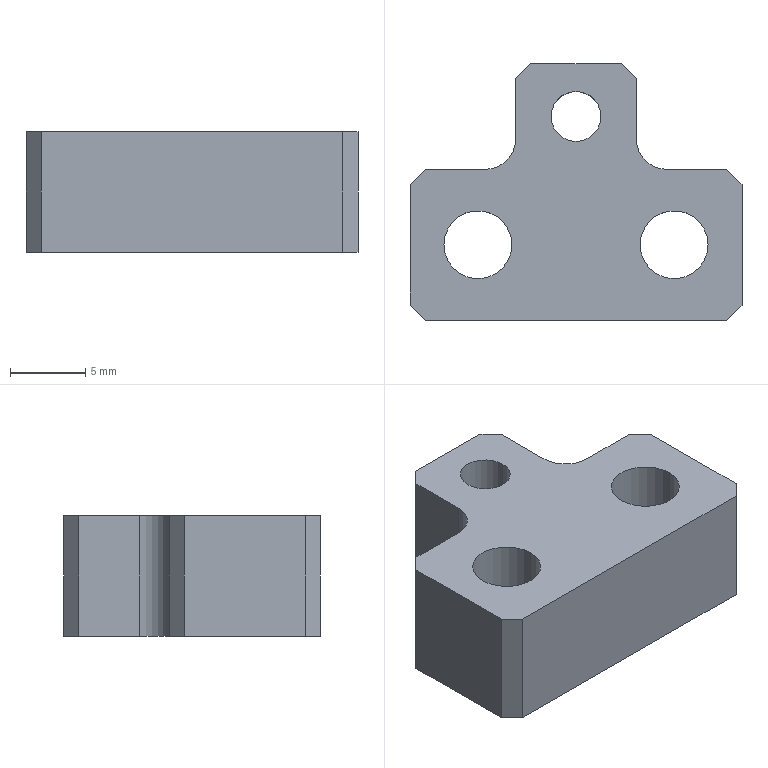Part | SolidWorks | features HoleWzd 2, Chamfer 1, Extrusion 1, Fillet 1, ICE 1 | 1 solid | 30 faces | box 22 x 17 x 8 mm | volume 1559 mm3 | plane 18 | cylinder 12 | commonest cylinder face diameters 4.5 x4 8 x4 3.3 x2 4 x2
STEP:
#1=CARTESIAN_POINT('',(1.65,8.5,8.));
#2=VERTEX_POINT('',#1);
#3=CARTESIAN_POINT('',(-1.65,8.5,8.));
#4=VERTEX_POINT('',#3);
#5=CARTESIAN_POINT('',(0.,8.5,8.));
#6=DIRECTION('',(0.,0.,-1.));
#7=DIRECTION('',(-1.,0.,0.));
#8=AXIS2_PLACEMENT_3D('',#5,#6,#7);
#9=CIRCLE('',#8,1.65);
#10=EDGE_CURVE('',#2,#4,#9,.T.);
#11=ORIENTED_EDGE('',*,*,#10,.F.);
#12=CARTESIAN_POINT('',(1.65,8.5,0.));
#13=VERTEX_POINT('',#12);
#14=CARTESIAN_POINT('',(1.65,8.5,0.));
#15=DIRECTION('',(0.,0.,-1.));
#16=VECTOR('',#15,1000.);
#17=LINE('',#14,#16);
#18=EDGE_CURVE('',#2,#13,#17,.T.);
#19=ORIENTED_EDGE('',*,*,#18,.T.);
#20=CARTESIAN_POINT('',(-1.65,8.5,0.));
#21=VERTEX_POINT('',#20);
#22=CARTESIAN_POINT('',(0.,8.5,0.));
#23=DIRECTION('',(0.,0.,-1.));
#24=DIRECTION('',(-1.,0.,0.));
#25=AXIS2_PLACEMENT_3D('',#22,#23,#24);
#26=CIRCLE('',#25,1.65);
#27=EDGE_CURVE('',#13,#21,#26,.T.);
#28=ORIENTED_EDGE('',*,*,#27,.T.);
#29=CARTESIAN_POINT('',(-1.65,8.5,0.));
#30=DIRECTION('',(0.,0.,-1.));
#31=VECTOR('',#30,1000.);
#32=LINE('',#29,#31);
#33=EDGE_CURVE('',#4,#21,#32,.T.);
#34=ORIENTED_EDGE('',*,*,#33,.F.);
#35=EDGE_LOOP('',(#11,#19,#28,#34));
#36=FACE_OUTER_BOUND('',#35,.T.);
#37=CARTESIAN_POINT('',(0.,8.5,0.));
#38=DIRECTION('',(0.,0.,-1.));
#39=DIRECTION('',(-1.,0.,0.));
#40=AXIS2_PLACEMENT_3D('',#37,#38,#39);
#41=CYLINDRICAL_SURFACE('',#40,1.65);
#42=ADVANCED_FACE('',(#36),#41,.F.);
#43=CARTESIAN_POINT('',(10.5,0.,4.6));
#44=VERTEX_POINT('',#43);
#45=CARTESIAN_POINT('',(2.5,0.,4.6));
#46=VERTEX_POINT('',#45);
#47=CARTESIAN_POINT('',(6.5,0.,4.6));
#48=DIRECTION('',(0.,0.,-1.));
#49=DIRECTION('',(-1.,0.,0.));
#50=AXIS2_PLACEMENT_3D('',#47,#48,#49);
#51=CIRCLE('',#50,4.);
#52=EDGE_CURVE('',#44,#46,#51,.T.);
#53=ORIENTED_EDGE('',*,*,#52,.F.);
#54=CARTESIAN_POINT('',(10.5,0.,0.));
#55=VERTEX_POINT('',#54);
#56=CARTESIAN_POINT('',(10.5,0.,0.));
#57=DIRECTION('',(0.,0.,-1.));
#58=VECTOR('',#57,1000.);
#59=LINE('',#56,#58);
#60=EDGE_CURVE('',#44,#55,#59,.T.);
#61=ORIENTED_EDGE('',*,*,#60,.T.);
#62=CARTESIAN_POINT('',(2.5,0.,0.));
#63=VERTEX_POINT('',#62);
#64=CARTESIAN_POINT('',(6.5,0.,0.));
#65=DIRECTION('',(0.,0.,-1.));
#66=DIRECTION('',(-1.,0.,0.));
#67=AXIS2_PLACEMENT_3D('',#64,#65,#66);
#68=CIRCLE('',#67,4.);
#69=EDGE_CURVE('',#55,#63,#68,.T.);
#70=ORIENTED_EDGE('',*,*,#69,.T.);
#71=CARTESIAN_POINT('',(2.5,0.,0.));
#72=DIRECTION('',(0.,0.,-1.));
#73=VECTOR('',#72,1000.);
#74=LINE('',#71,#73);
#75=EDGE_CURVE('',#46,#63,#74,.T.);
#76=ORIENTED_EDGE('',*,*,#75,.F.);
#77=EDGE_LOOP('',(#53,#61,#70,#76));
#78=FACE_OUTER_BOUND('',#77,.T.);
#79=CARTESIAN_POINT('',(6.5,0.,0.));
#80=DIRECTION('',(0.,0.,-1.));
#81=DIRECTION('',(-1.,0.,0.));
#82=AXIS2_PLACEMENT_3D('',#79,#80,#81);
#83=CYLINDRICAL_SURFACE('',#82,4.);
#84=ADVANCED_FACE('',(#78),#83,.F.);
#85=CARTESIAN_POINT('',(8.75,0.,8.));
#86=VERTEX_POINT('',#85);
#87=CARTESIAN_POINT('',(4.25,0.,8.));
#88=VERTEX_POINT('',#87);
#89=CARTESIAN_POINT('',(6.5,0.,8.));
#90=DIRECTION('',(0.,0.,-1.));
#91=DIRECTION('',(-1.,0.,0.));
#92=AXIS2_PLACEMENT_3D('',#89,#90,#91);
#93=CIRCLE('',#92,2.25);
#94=EDGE_CURVE('',#86,#88,#93,.T.);
#95=ORIENTED_EDGE('',*,*,#94,.F.);
#96=CARTESIAN_POINT('',(8.75,0.,4.6));
#97=VERTEX_POINT('',#96);
#98=CARTESIAN_POINT('',(8.75,0.,0.));
#99=DIRECTION('',(0.,0.,-1.));
#100=VECTOR('',#99,1000.);
#101=LINE('',#98,#100);
#102=EDGE_CURVE('',#86,#97,#101,.T.);
#103=ORIENTED_EDGE('',*,*,#102,.T.);
#104=CARTESIAN_POINT('',(4.25,0.,4.6));
#105=VERTEX_POINT('',#104);
#106=CARTESIAN_POINT('',(6.5,0.,4.6));
#107=DIRECTION('',(0.,0.,-1.));
#108=DIRECTION('',(-1.,0.,0.));
#109=AXIS2_PLACEMENT_3D('',#106,#107,#108);
#110=CIRCLE('',#109,2.25);
#111=EDGE_CURVE('',#97,#105,#110,.T.);
#112=ORIENTED_EDGE('',*,*,#111,.T.);
#113=CARTESIAN_POINT('',(4.25,0.,0.));
#114=DIRECTION('',(0.,0.,-1.));
#115=VECTOR('',#114,1000.);
#116=LINE('',#113,#115);
#117=EDGE_CURVE('',#88,#105,#116,.T.);
#118=ORIENTED_EDGE('',*,*,#117,.F.);
#119=EDGE_LOOP('',(#95,#103,#112,#118));
#120=FACE_OUTER_BOUND('',#119,.T.);
#121=CARTESIAN_POINT('',(6.5,0.,0.));
#122=DIRECTION('',(0.,0.,-1.));
#123=DIRECTION('',(-1.,0.,0.));
#124=AXIS2_PLACEMENT_3D('',#121,#122,#123);
#125=CYLINDRICAL_SURFACE('',#124,2.25);
#126=ADVANCED_FACE('',(#120),#125,.F.);
#127=CARTESIAN_POINT('',(-2.5,0.,4.6));
#128=VERTEX_POINT('',#127);
#129=CARTESIAN_POINT('',(-10.5,0.,4.6));
#130=VERTEX_POINT('',#129);
#131=CARTESIAN_POINT('',(-6.5,0.,4.6));
#132=DIRECTION('',(0.,0.,-1.));
#133=DIRECTION('',(-1.,0.,0.));
#134=AXIS2_PLACEMENT_3D('',#131,#132,#133);
#135=CIRCLE('',#134,4.);
#136=EDGE_CURVE('',#128,#130,#135,.T.);
#137=ORIENTED_EDGE('',*,*,#136,.F.);
#138=CARTESIAN_POINT('',(-2.5,0.,0.));
#139=VERTEX_POINT('',#138);
#140=CARTESIAN_POINT('',(-2.5,0.,0.));
#141=DIRECTION('',(0.,0.,-1.));
#142=VECTOR('',#141,1000.);
#143=LINE('',#140,#142);
#144=EDGE_CURVE('',#128,#139,#143,.T.);
#145=ORIENTED_EDGE('',*,*,#144,.T.);
#146=CARTESIAN_POINT('',(-10.5,0.,0.));
#147=VERTEX_POINT('',#146);
#148=CARTESIAN_POINT('',(-6.5,0.,0.));
#149=DIRECTION('',(0.,0.,-1.));
#150=DIRECTION('',(-1.,0.,0.));
#151=AXIS2_PLACEMENT_3D('',#148,#149,#150);
#152=CIRCLE('',#151,4.);
#153=EDGE_CURVE('',#139,#147,#152,.T.);
#154=ORIENTED_EDGE('',*,*,#153,.T.);
#155=CARTESIAN_POINT('',(-10.5,0.,0.));
#156=DIRECTION('',(0.,0.,-1.));
#157=VECTOR('',#156,1000.);
#158=LINE('',#155,#157);
#159=EDGE_CURVE('',#130,#147,#158,.T.);
#160=ORIENTED_EDGE('',*,*,#159,.F.);
#161=EDGE_LOOP('',(#137,#145,#154,#160));
#162=FACE_OUTER_BOUND('',#161,.T.);
#163=CARTESIAN_POINT('',(-6.5,0.,0.));
#164=DIRECTION('',(0.,0.,-1.));
#165=DIRECTION('',(-1.,0.,0.));
#166=AXIS2_PLACEMENT_3D('',#163,#164,#165);
#167=CYLINDRICAL_SURFACE('',#166,4.);
#168=ADVANCED_FACE('',(#162),#167,.F.);
#169=CARTESIAN_POINT('',(-4.25,0.,8.));
#170=VERTEX_POINT('',#169);
#171=CARTESIAN_POINT('',(-8.75,0.,8.));
#172=VERTEX_POINT('',#171);
#173=CARTESIAN_POINT('',(-6.5,0.,8.));
#174=DIRECTION('',(0.,0.,-1.));
#175=DIRECTION('',(-1.,0.,0.));
#176=AXIS2_PLACEMENT_3D('',#173,#174,#175);
#177=CIRCLE('',#176,2.25);
#178=EDGE_CURVE('',#170,#172,#177,.T.);
#179=ORIENTED_EDGE('',*,*,#178,.F.);
#180=CARTESIAN_POINT('',(-4.25,0.,4.6));
#181=VERTEX_POINT('',#180);
#182=CARTESIAN_POINT('',(-4.25,0.,0.));
#183=DIRECTION('',(0.,0.,-1.));
#184=VECTOR('',#183,1000.);
#185=LINE('',#182,#184);
#186=EDGE_CURVE('',#170,#181,#185,.T.);
#187=ORIENTED_EDGE('',*,*,#186,.T.);
#188=CARTESIAN_POINT('',(-8.75,0.,4.6));
#189=VERTEX_POINT('',#188);
#190=CARTESIAN_POINT('',(-6.5,0.,4.6));
#191=DIRECTION('',(0.,0.,-1.));
#192=DIRECTION('',(-1.,0.,0.));
#193=AXIS2_PLACEMENT_3D('',#190,#191,#192);
#194=CIRCLE('',#193,2.25);
#195=EDGE_CURVE('',#181,#189,#194,.T.);
#196=ORIENTED_EDGE('',*,*,#195,.T.);
#197=CARTESIAN_POINT('',(-8.75,0.,0.));
#198=DIRECTION('',(0.,0.,-1.));
#199=VECTOR('',#198,1000.);
#200=LINE('',#197,#199);
#201=EDGE_CURVE('',#172,#189,#200,.T.);
#202=ORIENTED_EDGE('',*,*,#201,.F.);
#203=EDGE_LOOP('',(#179,#187,#196,#202));
#204=FACE_OUTER_BOUND('',#203,.T.);
#205=CARTESIAN_POINT('',(-6.5,0.,0.));
#206=DIRECTION('',(0.,0.,-1.));
#207=DIRECTION('',(-1.,0.,0.));
#208=AXIS2_PLACEMENT_3D('',#205,#206,#207);
#209=CYLINDRICAL_SURFACE('',#208,2.25);
#210=ADVANCED_FACE('',(#204),#209,.F.);
#211=CARTESIAN_POINT('',(10.,5.,8.));
#212=VERTEX_POINT('',#211);
#213=CARTESIAN_POINT('',(6.,5.,8.));
#214=VERTEX_POINT('',#213);
#215=CARTESIAN_POINT('',(-11.,5.,8.));
#216=DIRECTION('',(-1.,0.,0.));
#217=VECTOR('',#216,1000.);
#218=LINE('',#215,#217);
#219=EDGE_CURVE('',#212,#214,#218,.T.);
#220=ORIENTED_EDGE('',*,*,#219,.F.);
#221=CARTESIAN_POINT('',(10.,5.,0.));
#222=VERTEX_POINT('',#221);
#223=CARTESIAN_POINT('',(10.,5.,8.));
#224=DIRECTION('',(0.,0.,-1.));
#225=VECTOR('',#224,1000.);
#226=LINE('',#223,#225);
#227=EDGE_CURVE('',#212,#222,#226,.T.);
#228=ORIENTED_EDGE('',*,*,#227,.T.);
#229=CARTESIAN_POINT('',(6.,5.,0.));
#230=VERTEX_POINT('',#229);
#231=CARTESIAN_POINT('',(-11.,5.,0.));
#232=DIRECTION('',(-1.,0.,0.));
#233=VECTOR('',#232,1000.);
#234=LINE('',#231,#233);
#235=EDGE_CURVE('',#222,#230,#234,.T.);
#236=ORIENTED_EDGE('',*,*,#235,.T.);
#237=CARTESIAN_POINT('',(6.,5.,8.));
#238=DIRECTION('',(0.,0.,1.));
#239=VECTOR('',#238,1000.);
#240=LINE('',#237,#239);
#241=EDGE_CURVE('',#230,#214,#240,.T.);
#242=ORIENTED_EDGE('',*,*,#241,.T.);
#243=EDGE_LOOP('',(#220,#228,#236,#242));
#244=FACE_OUTER_BOUND('',#243,.T.);
#245=CARTESIAN_POINT('',(-11.,5.,8.));
#246=DIRECTION('',(0.,-1.,0.));
#247=DIRECTION('',(0.,0.,-1.));
#248=AXIS2_PLACEMENT_3D('',#245,#246,#247);
#249=PLANE('',#248);
#250=ADVANCED_FACE('',(#244),#249,.F.);
#251=CARTESIAN_POINT('',(11.,-4.,8.));
#252=VERTEX_POINT('',#251);
#253=CARTESIAN_POINT('',(11.,4.,8.));
#254=VERTEX_POINT('',#253);
#255=CARTESIAN_POINT('',(11.,5.,8.));
#256=DIRECTION('',(0.,1.,0.));
#257=VECTOR('',#256,1000.);
#258=LINE('',#255,#257);
#259=EDGE_CURVE('',#252,#254,#258,.T.);
#260=ORIENTED_EDGE('',*,*,#259,.F.);
#261=CARTESIAN_POINT('',(11.,-4.,0.));
#262=VERTEX_POINT('',#261);
#263=CARTESIAN_POINT('',(11.,-4.,8.));
#264=DIRECTION('',(0.,0.,-1.));
#265=VECTOR('',#264,1000.);
#266=LINE('',#263,#265);
#267=EDGE_CURVE('',#252,#262,#266,.T.);
#268=ORIENTED_EDGE('',*,*,#267,.T.);
#269=CARTESIAN_POINT('',(11.,4.,0.));
#270=VERTEX_POINT('',#269);
#271=CARTESIAN_POINT('',(11.,5.,0.));
#272=DIRECTION('',(0.,1.,0.));
#273=VECTOR('',#272,1000.);
#274=LINE('',#271,#273);
#275=EDGE_CURVE('',#262,#270,#274,.T.);
#276=ORIENTED_EDGE('',*,*,#275,.T.);
#277=CARTESIAN_POINT('',(11.,4.,8.));
#278=DIRECTION('',(0.,0.,1.));
#279=VECTOR('',#278,1000.);
#280=LINE('',#277,#279);
#281=EDGE_CURVE('',#270,#254,#280,.T.);
#282=ORIENTED_EDGE('',*,*,#281,.T.);
#283=EDGE_LOOP('',(#260,#268,#276,#282));
#284=FACE_OUTER_BOUND('',#283,.T.);
#285=CARTESIAN_POINT('',(11.,5.,8.));
#286=DIRECTION('',(-1.,0.,0.));
#287=DIRECTION('',(0.,0.,1.));
#288=AXIS2_PLACEMENT_3D('',#285,#286,#287);
#289=PLANE('',#288);
#290=ADVANCED_FACE('',(#284),#289,.F.);
#291=CARTESIAN_POINT('',(-6.,5.,0.));
#292=VERTEX_POINT('',#291);
#293=CARTESIAN_POINT('',(-10.,5.,0.));
#294=VERTEX_POINT('',#293);
#295=CARTESIAN_POINT('',(-11.,5.,0.));
#296=DIRECTION('',(-1.,0.,0.));
#297=VECTOR('',#296,1000.);
#298=LINE('',#295,#297);
#299=EDGE_CURVE('',#292,#294,#298,.T.);
#300=ORIENTED_EDGE('',*,*,#299,.T.);
#301=CARTESIAN_POINT('',(-10.,5.,8.));
#302=VERTEX_POINT('',#301);
#303=CARTESIAN_POINT('',(-10.,5.,8.));
#304=DIRECTION('',(0.,0.,1.));
#305=VECTOR('',#304,1000.);
#306=LINE('',#303,#305);
#307=EDGE_CURVE('',#294,#302,#306,.T.);
#308=ORIENTED_EDGE('',*,*,#307,.T.);
#309=CARTESIAN_POINT('',(-6.,5.,8.));
#310=VERTEX_POINT('',#309);
#311=CARTESIAN_POINT('',(-11.,5.,8.));
#312=DIRECTION('',(-1.,0.,0.));
#313=VECTOR('',#312,1000.);
#314=LINE('',#311,#313);
#315=EDGE_CURVE('',#310,#302,#314,.T.);
#316=ORIENTED_EDGE('',*,*,#315,.F.);
#317=CARTESIAN_POINT('',(-6.,5.,8.));
#318=DIRECTION('',(0.,0.,-1.));
#319=VECTOR('',#318,1000.);
#320=LINE('',#317,#319);
#321=EDGE_CURVE('',#310,#292,#320,.T.);
#322=ORIENTED_EDGE('',*,*,#321,.T.);
#323=EDGE_LOOP('',(#300,#308,#316,#322));
#324=FACE_OUTER_BOUND('',#323,.T.);
#325=CARTESIAN_POINT('',(-11.,5.,8.));
#326=DIRECTION('',(0.,-1.,0.));
#327=DIRECTION('',(0.,0.,-1.));
#328=AXIS2_PLACEMENT_3D('',#325,#326,#327);
#329=PLANE('',#328);
#330=ADVANCED_FACE('',(#324),#329,.F.);
#331=CARTESIAN_POINT('',(-11.,4.,8.));
#332=VERTEX_POINT('',#331);
#333=CARTESIAN_POINT('',(-11.,-4.,8.));
#334=VERTEX_POINT('',#333);
#335=CARTESIAN_POINT('',(-11.,5.,8.));
#336=DIRECTION('',(0.,-1.,0.));
#337=VECTOR('',#336,1000.);
#338=LINE('',#335,#337);
#339=EDGE_CURVE('',#332,#334,#338,.T.);
#340=ORIENTED_EDGE('',*,*,#339,.F.);
#341=CARTESIAN_POINT('',(-11.,4.,0.));
#342=VERTEX_POINT('',#341);
#343=CARTESIAN_POINT('',(-11.,4.,8.));
#344=DIRECTION('',(0.,0.,-1.));
#345=VECTOR('',#344,1000.);
#346=LINE('',#343,#345);
#347=EDGE_CURVE('',#332,#342,#346,.T.);
#348=ORIENTED_EDGE('',*,*,#347,.T.);
#349=CARTESIAN_POINT('',(-11.,-4.,0.));
#350=VERTEX_POINT('',#349);
#351=CARTESIAN_POINT('',(-11.,5.,0.));
#352=DIRECTION('',(0.,-1.,0.));
#353=VECTOR('',#352,1000.);
#354=LINE('',#351,#353);
#355=EDGE_CURVE('',#342,#350,#354,.T.);
#356=ORIENTED_EDGE('',*,*,#355,.T.);
#357=CARTESIAN_POINT('',(-11.,-4.,8.));
#358=DIRECTION('',(0.,0.,1.));
#359=VECTOR('',#358,1000.);
#360=LINE('',#357,#359);
#361=EDGE_CURVE('',#350,#334,#360,.T.);
#362=ORIENTED_EDGE('',*,*,#361,.T.);
#363=EDGE_LOOP('',(#340,#348,#356,#362));
#364=FACE_OUTER_BOUND('',#363,.T.);
#365=CARTESIAN_POINT('',(-11.,5.,8.));
#366=DIRECTION('',(1.,0.,0.));
#367=DIRECTION('',(0.,1.,0.));
#368=AXIS2_PLACEMENT_3D('',#365,#366,#367);
#369=PLANE('',#368);
#370=ADVANCED_FACE('',(#364),#369,.F.);
#371=CARTESIAN_POINT('',(-10.,-5.,0.));
#372=VERTEX_POINT('',#371);
#373=CARTESIAN_POINT('',(10.,-5.,0.));
#374=VERTEX_POINT('',#373);
#375=CARTESIAN_POINT('',(-11.,-5.,0.));
#376=DIRECTION('',(1.,0.,0.));
#377=VECTOR('',#376,1000.);
#378=LINE('',#375,#377);
#379=EDGE_CURVE('',#372,#374,#378,.T.);
#380=ORIENTED_EDGE('',*,*,#379,.T.);
#381=CARTESIAN_POINT('',(10.,-5.,8.));
#382=VERTEX_POINT('',#381);
#383=CARTESIAN_POINT('',(10.,-5.,8.));
#384=DIRECTION('',(0.,0.,1.));
#385=VECTOR('',#384,1000.);
#386=LINE('',#383,#385);
#387=EDGE_CURVE('',#374,#382,#386,.T.);
#388=ORIENTED_EDGE('',*,*,#387,.T.);
#389=CARTESIAN_POINT('',(-10.,-5.,8.));
#390=VERTEX_POINT('',#389);
#391=CARTESIAN_POINT('',(-11.,-5.,8.));
#392=DIRECTION('',(1.,0.,0.));
#393=VECTOR('',#392,1000.);
#394=LINE('',#391,#393);
#395=EDGE_CURVE('',#390,#382,#394,.T.);
#396=ORIENTED_EDGE('',*,*,#395,.F.);
#397=CARTESIAN_POINT('',(-10.,-5.,8.));
#398=DIRECTION('',(0.,0.,-1.));
#399=VECTOR('',#398,1000.);
#400=LINE('',#397,#399);
#401=EDGE_CURVE('',#390,#372,#400,.T.);
#402=ORIENTED_EDGE('',*,*,#401,.T.);
#403=EDGE_LOOP('',(#380,#388,#396,#402));
#404=FACE_OUTER_BOUND('',#403,.T.);
#405=CARTESIAN_POINT('',(-11.,-5.,8.));
#406=DIRECTION('',(0.,1.,0.));
#407=DIRECTION('',(0.,0.,1.));
#408=AXIS2_PLACEMENT_3D('',#405,#406,#407);
#409=PLANE('',#408);
#410=ADVANCED_FACE('',(#404),#409,.F.);
#411=CARTESIAN_POINT('',(0.,8.5,8.));
#412=DIRECTION('',(0.,0.,-1.));
#413=DIRECTION('',(-1.,0.,0.));
#414=AXIS2_PLACEMENT_3D('',#411,#412,#413);
#415=CIRCLE('',#414,1.65);
#416=EDGE_CURVE('',#4,#2,#415,.T.);
#417=ORIENTED_EDGE('',*,*,#416,.T.);
#418=ORIENTED_EDGE('',*,*,#10,.T.);
#419=EDGE_LOOP('',(#417,#418));
#420=FACE_BOUND('',#419,.T.);
#421=CARTESIAN_POINT('',(6.5,0.,8.));
#422=DIRECTION('',(0.,0.,-1.));
#423=DIRECTION('',(-1.,0.,0.));
#424=AXIS2_PLACEMENT_3D('',#421,#422,#423);
#425=CIRCLE('',#424,2.25);
#426=EDGE_CURVE('',#88,#86,#425,.T.);
#427=ORIENTED_EDGE('',*,*,#426,.T.);
#428=ORIENTED_EDGE('',*,*,#94,.T.);
#429=EDGE_LOOP('',(#427,#428));
#430=FACE_BOUND('',#429,.T.);
#431=CARTESIAN_POINT('',(-6.5,0.,8.));
#432=DIRECTION('',(0.,0.,-1.));
#433=DIRECTION('',(-1.,0.,0.));
#434=AXIS2_PLACEMENT_3D('',#431,#432,#433);
#435=CIRCLE('',#434,2.25);
#436=EDGE_CURVE('',#172,#170,#435,.T.);
#437=ORIENTED_EDGE('',*,*,#436,.T.);
#438=ORIENTED_EDGE('',*,*,#178,.T.);
#439=EDGE_LOOP('',(#437,#438));
#440=FACE_BOUND('',#439,.T.);
#441=ORIENTED_EDGE('',*,*,#395,.T.);
#442=CARTESIAN_POINT('',(7.5,-7.5,8.));
#443=DIRECTION('',(0.7071,0.7071,0.));
#444=VECTOR('',#443,1000.);
#445=LINE('',#442,#444);
#446=EDGE_CURVE('',#382,#252,#445,.T.);
#447=ORIENTED_EDGE('',*,*,#446,.T.);
#448=ORIENTED_EDGE('',*,*,#259,.T.);
#449=CARTESIAN_POINT('',(7.5,7.5,8.));
#450=DIRECTION('',(-0.7071,0.7071,0.));
#451=VECTOR('',#450,1000.);
#452=LINE('',#449,#451);
#453=EDGE_CURVE('',#254,#212,#452,.T.);
#454=ORIENTED_EDGE('',*,*,#453,.T.);
#455=ORIENTED_EDGE('',*,*,#219,.T.);
#456=CARTESIAN_POINT('',(4.,7.,8.));
#457=VERTEX_POINT('',#456);
#458=CARTESIAN_POINT('',(6.,7.,8.));
#459=DIRECTION('',(0.,0.,-1.));
#460=DIRECTION('',(1.,0.,0.));
#461=AXIS2_PLACEMENT_3D('',#458,#459,#460);
#462=CIRCLE('',#461,2.);
#463=EDGE_CURVE('',#214,#457,#462,.T.);
#464=ORIENTED_EDGE('',*,*,#463,.T.);
#465=CARTESIAN_POINT('',(4.,11.,8.));
#466=VERTEX_POINT('',#465);
#467=CARTESIAN_POINT('',(4.,5.,8.));
#468=DIRECTION('',(0.,-1.,0.));
#469=VECTOR('',#468,1000.);
#470=LINE('',#467,#469);
#471=EDGE_CURVE('',#466,#457,#470,.T.);
#472=ORIENTED_EDGE('',*,*,#471,.F.);
#473=CARTESIAN_POINT('',(3.,12.,8.));
#474=VERTEX_POINT('',#473);
#475=CARTESIAN_POINT('',(7.5,7.5,8.));
#476=DIRECTION('',(-0.7071,0.7071,0.));
#477=VECTOR('',#476,1000.);
#478=LINE('',#475,#477);
#479=EDGE_CURVE('',#466,#474,#478,.T.);
#480=ORIENTED_EDGE('',*,*,#479,.T.);
#481=CARTESIAN_POINT('',(-3.,12.,8.));
#482=VERTEX_POINT('',#481);
#483=CARTESIAN_POINT('',(4.,12.,8.));
#484=DIRECTION('',(1.,0.,0.));
#485=VECTOR('',#484,1000.);
#486=LINE('',#483,#485);
#487=EDGE_CURVE('',#482,#474,#486,.T.);
#488=ORIENTED_EDGE('',*,*,#487,.F.);
#489=CARTESIAN_POINT('',(-4.,11.,8.));
#490=VERTEX_POINT('',#489);
#491=CARTESIAN_POINT('',(-7.5,7.5,8.));
#492=DIRECTION('',(-0.7071,-0.7071,0.));
#493=VECTOR('',#492,1000.);
#494=LINE('',#491,#493);
#495=EDGE_CURVE('',#482,#490,#494,.T.);
#496=ORIENTED_EDGE('',*,*,#495,.T.);
#497=CARTESIAN_POINT('',(-4.,7.,8.));
#498=VERTEX_POINT('',#497);
#499=CARTESIAN_POINT('',(-4.,5.,8.));
#500=DIRECTION('',(0.,1.,0.));
#501=VECTOR('',#500,1000.);
#502=LINE('',#499,#501);
#503=EDGE_CURVE('',#498,#490,#502,.T.);
#504=ORIENTED_EDGE('',*,*,#503,.F.);
#505=CARTESIAN_POINT('',(-6.,7.,8.));
#506=DIRECTION('',(0.,0.,-1.));
#507=DIRECTION('',(1.,0.,0.));
#508=AXIS2_PLACEMENT_3D('',#505,#506,#507);
#509=CIRCLE('',#508,2.);
#510=EDGE_CURVE('',#498,#310,#509,.T.);
#511=ORIENTED_EDGE('',*,*,#510,.T.);
#512=ORIENTED_EDGE('',*,*,#315,.T.);
#513=CARTESIAN_POINT('',(-7.5,7.5,8.));
#514=DIRECTION('',(-0.7071,-0.7071,0.));
#515=VECTOR('',#514,1000.);
#516=LINE('',#513,#515);
#517=EDGE_CURVE('',#302,#332,#516,.T.);
#518=ORIENTED_EDGE('',*,*,#517,.T.);
#519=ORIENTED_EDGE('',*,*,#339,.T.);
#520=CARTESIAN_POINT('',(-7.5,-7.5,8.));
#521=DIRECTION('',(0.7071,-0.7071,0.));
#522=VECTOR('',#521,1000.);
#523=LINE('',#520,#522);
#524=EDGE_CURVE('',#334,#390,#523,.T.);
#525=ORIENTED_EDGE('',*,*,#524,.T.);
#526=EDGE_LOOP('',(#441,#447,#448,#454,#455,#464,#472,#480,#488,#496,#504,#511,#512,#518,#519,#525));
#527=FACE_OUTER_BOUND('',#526,.T.);
#528=CARTESIAN_POINT('',(0.,0.,8.));
#529=DIRECTION('',(0.,0.,1.));
#530=DIRECTION('',(1.,0.,0.));
#531=AXIS2_PLACEMENT_3D('',#528,#529,#530);
#532=PLANE('',#531);
#533=ADVANCED_FACE('',(#420,#430,#440,#527),#532,.T.);
#534=CARTESIAN_POINT('',(0.,8.5,0.));
#535=DIRECTION('',(0.,0.,-1.));
#536=DIRECTION('',(-1.,0.,0.));
#537=AXIS2_PLACEMENT_3D('',#534,#535,#536);
#538=CIRCLE('',#537,1.65);
#539=EDGE_CURVE('',#21,#13,#538,.T.);
#540=ORIENTED_EDGE('',*,*,#539,.F.);
#541=ORIENTED_EDGE('',*,*,#27,.F.);
#542=EDGE_LOOP('',(#540,#541));
#543=FACE_BOUND('',#542,.T.);
#544=CARTESIAN_POINT('',(6.5,0.,0.));
#545=DIRECTION('',(0.,0.,-1.));
#546=DIRECTION('',(-1.,0.,0.));
#547=AXIS2_PLACEMENT_3D('',#544,#545,#546);
#548=CIRCLE('',#547,4.);
#549=EDGE_CURVE('',#63,#55,#548,.T.);
#550=ORIENTED_EDGE('',*,*,#549,.F.);
#551=ORIENTED_EDGE('',*,*,#69,.F.);
#552=EDGE_LOOP('',(#550,#551));
#553=FACE_BOUND('',#552,.T.);
#554=CARTESIAN_POINT('',(-6.5,0.,0.));
#555=DIRECTION('',(0.,0.,-1.));
#556=DIRECTION('',(-1.,0.,0.));
#557=AXIS2_PLACEMENT_3D('',#554,#555,#556);
#558=CIRCLE('',#557,4.);
#559=EDGE_CURVE('',#147,#139,#558,.T.);
#560=ORIENTED_EDGE('',*,*,#559,.F.);
#561=ORIENTED_EDGE('',*,*,#153,.F.);
#562=EDGE_LOOP('',(#560,#561));
#563=FACE_BOUND('',#562,.T.);
#564=ORIENTED_EDGE('',*,*,#275,.F.);
#565=CARTESIAN_POINT('',(11.,-4.,0.));
#566=DIRECTION('',(-0.7071,-0.7071,0.));
#567=VECTOR('',#566,1000.);
#568=LINE('',#565,#567);
#569=EDGE_CURVE('',#262,#374,#568,.T.);
#570=ORIENTED_EDGE('',*,*,#569,.T.);
#571=ORIENTED_EDGE('',*,*,#379,.F.);
#572=CARTESIAN_POINT('',(-10.,-5.,0.));
#573=DIRECTION('',(-0.7071,0.7071,0.));
#574=VECTOR('',#573,1000.);
#575=LINE('',#572,#574);
#576=EDGE_CURVE('',#372,#350,#575,.T.);
#577=ORIENTED_EDGE('',*,*,#576,.T.);
#578=ORIENTED_EDGE('',*,*,#355,.F.);
#579=CARTESIAN_POINT('',(-11.,4.,0.));
#580=DIRECTION('',(0.7071,0.7071,0.));
#581=VECTOR('',#580,1000.);
#582=LINE('',#579,#581);
#583=EDGE_CURVE('',#342,#294,#582,.T.);
#584=ORIENTED_EDGE('',*,*,#583,.T.);
#585=ORIENTED_EDGE('',*,*,#299,.F.);
#586=CARTESIAN_POINT('',(-4.,7.,0.));
#587=VERTEX_POINT('',#586);
#588=CARTESIAN_POINT('',(-6.,7.,0.));
#589=DIRECTION('',(0.,0.,1.));
#590=DIRECTION('',(1.,0.,0.));
#591=AXIS2_PLACEMENT_3D('',#588,#589,#590);
#592=CIRCLE('',#591,2.);
#593=EDGE_CURVE('',#292,#587,#592,.T.);
#594=ORIENTED_EDGE('',*,*,#593,.T.);
#595=CARTESIAN_POINT('',(-4.,11.,0.));
#596=VERTEX_POINT('',#595);
#597=CARTESIAN_POINT('',(-4.,5.,0.));
#598=DIRECTION('',(0.,1.,0.));
#599=VECTOR('',#598,1000.);
#600=LINE('',#597,#599);
#601=EDGE_CURVE('',#587,#596,#600,.T.);
#602=ORIENTED_EDGE('',*,*,#601,.T.);
#603=CARTESIAN_POINT('',(-3.,12.,0.));
#604=VERTEX_POINT('',#603);
#605=CARTESIAN_POINT('',(-4.,11.,0.));
#606=DIRECTION('',(0.7071,0.7071,0.));
#607=VECTOR('',#606,1000.);
#608=LINE('',#605,#607);
#609=EDGE_CURVE('',#596,#604,#608,.T.);
#610=ORIENTED_EDGE('',*,*,#609,.T.);
#611=CARTESIAN_POINT('',(3.,12.,0.));
#612=VERTEX_POINT('',#611);
#613=CARTESIAN_POINT('',(4.,12.,0.));
#614=DIRECTION('',(1.,0.,0.));
#615=VECTOR('',#614,1000.);
#616=LINE('',#613,#615);
#617=EDGE_CURVE('',#604,#612,#616,.T.);
#618=ORIENTED_EDGE('',*,*,#617,.T.);
#619=CARTESIAN_POINT('',(4.,11.,0.));
#620=VERTEX_POINT('',#619);
#621=CARTESIAN_POINT('',(3.,12.,0.));
#622=DIRECTION('',(0.7071,-0.7071,0.));
#623=VECTOR('',#622,1000.);
#624=LINE('',#621,#623);
#625=EDGE_CURVE('',#612,#620,#624,.T.);
#626=ORIENTED_EDGE('',*,*,#625,.T.);
#627=CARTESIAN_POINT('',(4.,7.,0.));
#628=VERTEX_POINT('',#627);
#629=CARTESIAN_POINT('',(4.,5.,0.));
#630=DIRECTION('',(0.,-1.,0.));
#631=VECTOR('',#630,1000.);
#632=LINE('',#629,#631);
#633=EDGE_CURVE('',#620,#628,#632,.T.);
#634=ORIENTED_EDGE('',*,*,#633,.T.);
#635=CARTESIAN_POINT('',(6.,7.,0.));
#636=DIRECTION('',(0.,0.,1.));
#637=DIRECTION('',(1.,0.,0.));
#638=AXIS2_PLACEMENT_3D('',#635,#636,#637);
#639=CIRCLE('',#638,2.);
#640=EDGE_CURVE('',#628,#230,#639,.T.);
#641=ORIENTED_EDGE('',*,*,#640,.T.);
#642=ORIENTED_EDGE('',*,*,#235,.F.);
#643=CARTESIAN_POINT('',(10.,5.,0.));
#644=DIRECTION('',(0.7071,-0.7071,0.));
#645=VECTOR('',#644,1000.);
#646=LINE('',#643,#645);
#647=EDGE_CURVE('',#222,#270,#646,.T.);
#648=ORIENTED_EDGE('',*,*,#647,.T.);
#649=EDGE_LOOP('',(#564,#570,#571,#577,#578,#584,#585,#594,#602,#610,#618,#626,#634,#641,#642,#648));
#650=FACE_OUTER_BOUND('',#649,.T.);
#651=CARTESIAN_POINT('',(0.,0.,0.));
#652=DIRECTION('',(0.,0.,1.));
#653=DIRECTION('',(1.,0.,0.));
#654=AXIS2_PLACEMENT_3D('',#651,#652,#653);
#655=PLANE('',#654);
#656=ADVANCED_FACE('',(#543,#553,#563,#650),#655,.F.);
#657=ORIENTED_EDGE('',*,*,#186,.F.);
#658=ORIENTED_EDGE('',*,*,#436,.F.);
#659=ORIENTED_EDGE('',*,*,#201,.T.);
#660=CARTESIAN_POINT('',(-6.5,0.,4.6));
#661=DIRECTION('',(0.,0.,-1.));
#662=DIRECTION('',(-1.,0.,0.));
#663=AXIS2_PLACEMENT_3D('',#660,#661,#662);
#664=CIRCLE('',#663,2.25);
#665=EDGE_CURVE('',#189,#181,#664,.T.);
#666=ORIENTED_EDGE('',*,*,#665,.T.);
#667=EDGE_LOOP('',(#657,#658,#659,#666));
#668=FACE_OUTER_BOUND('',#667,.T.);
#669=CARTESIAN_POINT('',(-6.5,0.,0.));
#670=DIRECTION('',(0.,0.,-1.));
#671=DIRECTION('',(-1.,0.,0.));
#672=AXIS2_PLACEMENT_3D('',#669,#670,#671);
#673=CYLINDRICAL_SURFACE('',#672,2.25);
#674=ADVANCED_FACE('',(#668),#673,.F.);
#675=ORIENTED_EDGE('',*,*,#665,.F.);
#676=ORIENTED_EDGE('',*,*,#195,.F.);
#677=EDGE_LOOP('',(#675,#676));
#678=FACE_BOUND('',#677,.T.);
#679=CARTESIAN_POINT('',(-6.5,0.,4.6));
#680=DIRECTION('',(0.,0.,-1.));
#681=DIRECTION('',(-1.,0.,0.));
#682=AXIS2_PLACEMENT_3D('',#679,#680,#681);
#683=CIRCLE('',#682,4.);
#684=EDGE_CURVE('',#130,#128,#683,.T.);
#685=ORIENTED_EDGE('',*,*,#684,.T.);
#686=ORIENTED_EDGE('',*,*,#136,.T.);
#687=EDGE_LOOP('',(#685,#686));
#688=FACE_OUTER_BOUND('',#687,.T.);
#689=CARTESIAN_POINT('',(-4.25,0.,4.6));
#690=DIRECTION('',(0.,0.,1.));
#691=DIRECTION('',(1.,0.,0.));
#692=AXIS2_PLACEMENT_3D('',#689,#690,#691);
#693=PLANE('',#692);
#694=ADVANCED_FACE('',(#678,#688),#693,.F.);
#695=ORIENTED_EDGE('',*,*,#144,.F.);
#696=ORIENTED_EDGE('',*,*,#684,.F.);
#697=ORIENTED_EDGE('',*,*,#159,.T.);
#698=ORIENTED_EDGE('',*,*,#559,.T.);
#699=EDGE_LOOP('',(#695,#696,#697,#698));
#700=FACE_OUTER_BOUND('',#699,.T.);
#701=CARTESIAN_POINT('',(-6.5,0.,0.));
#702=DIRECTION('',(0.,0.,-1.));
#703=DIRECTION('',(-1.,0.,0.));
#704=AXIS2_PLACEMENT_3D('',#701,#702,#703);
#705=CYLINDRICAL_SURFACE('',#704,4.);
#706=ADVANCED_FACE('',(#700),#705,.F.);
#707=ORIENTED_EDGE('',*,*,#102,.F.);
#708=ORIENTED_EDGE('',*,*,#426,.F.);
#709=ORIENTED_EDGE('',*,*,#117,.T.);
#710=CARTESIAN_POINT('',(6.5,0.,4.6));
#711=DIRECTION('',(0.,0.,-1.));
#712=DIRECTION('',(-1.,0.,0.));
#713=AXIS2_PLACEMENT_3D('',#710,#711,#712);
#714=CIRCLE('',#713,2.25);
#715=EDGE_CURVE('',#105,#97,#714,.T.);
#716=ORIENTED_EDGE('',*,*,#715,.T.);
#717=EDGE_LOOP('',(#707,#708,#709,#716));
#718=FACE_OUTER_BOUND('',#717,.T.);
#719=CARTESIAN_POINT('',(6.5,0.,0.));
#720=DIRECTION('',(0.,0.,-1.));
#721=DIRECTION('',(-1.,0.,0.));
#722=AXIS2_PLACEMENT_3D('',#719,#720,#721);
#723=CYLINDRICAL_SURFACE('',#722,2.25);
#724=ADVANCED_FACE('',(#718),#723,.F.);
#725=ORIENTED_EDGE('',*,*,#715,.F.);
#726=ORIENTED_EDGE('',*,*,#111,.F.);
#727=EDGE_LOOP('',(#725,#726));
#728=FACE_BOUND('',#727,.T.);
#729=CARTESIAN_POINT('',(6.5,0.,4.6));
#730=DIRECTION('',(0.,0.,-1.));
#731=DIRECTION('',(-1.,0.,0.));
#732=AXIS2_PLACEMENT_3D('',#729,#730,#731);
#733=CIRCLE('',#732,4.);
#734=EDGE_CURVE('',#46,#44,#733,.T.);
#735=ORIENTED_EDGE('',*,*,#734,.T.);
#736=ORIENTED_EDGE('',*,*,#52,.T.);
#737=EDGE_LOOP('',(#735,#736));
#738=FACE_OUTER_BOUND('',#737,.T.);
#739=CARTESIAN_POINT('',(8.75,0.,4.6));
#740=DIRECTION('',(0.,0.,1.));
#741=DIRECTION('',(1.,0.,0.));
#742=AXIS2_PLACEMENT_3D('',#739,#740,#741);
#743=PLANE('',#742);
#744=ADVANCED_FACE('',(#728,#738),#743,.F.);
#745=ORIENTED_EDGE('',*,*,#60,.F.);
#746=ORIENTED_EDGE('',*,*,#734,.F.);
#747=ORIENTED_EDGE('',*,*,#75,.T.);
#748=ORIENTED_EDGE('',*,*,#549,.T.);
#749=EDGE_LOOP('',(#745,#746,#747,#748));
#750=FACE_OUTER_BOUND('',#749,.T.);
#751=CARTESIAN_POINT('',(6.5,0.,0.));
#752=DIRECTION('',(0.,0.,-1.));
#753=DIRECTION('',(-1.,0.,0.));
#754=AXIS2_PLACEMENT_3D('',#751,#752,#753);
#755=CYLINDRICAL_SURFACE('',#754,4.);
#756=ADVANCED_FACE('',(#750),#755,.F.);
#757=ORIENTED_EDGE('',*,*,#633,.F.);
#758=CARTESIAN_POINT('',(4.,11.,8.));
#759=DIRECTION('',(0.,0.,1.));
#760=VECTOR('',#759,1000.);
#761=LINE('',#758,#760);
#762=EDGE_CURVE('',#620,#466,#761,.T.);
#763=ORIENTED_EDGE('',*,*,#762,.T.);
#764=ORIENTED_EDGE('',*,*,#471,.T.);
#765=CARTESIAN_POINT('',(4.,7.,8.));
#766=DIRECTION('',(0.,0.,-1.));
#767=VECTOR('',#766,1000.);
#768=LINE('',#765,#767);
#769=EDGE_CURVE('',#457,#628,#768,.T.);
#770=ORIENTED_EDGE('',*,*,#769,.T.);
#771=EDGE_LOOP('',(#757,#763,#764,#770));
#772=FACE_OUTER_BOUND('',#771,.T.);
#773=CARTESIAN_POINT('',(4.,5.,8.));
#774=DIRECTION('',(1.,0.,0.));
#775=DIRECTION('',(0.,0.,-1.));
#776=AXIS2_PLACEMENT_3D('',#773,#774,#775);
#777=PLANE('',#776);
#778=ADVANCED_FACE('',(#772),#777,.T.);
#779=ORIENTED_EDGE('',*,*,#487,.T.);
#780=CARTESIAN_POINT('',(3.,12.,8.));
#781=DIRECTION('',(0.,0.,-1.));
#782=VECTOR('',#781,1000.);
#783=LINE('',#780,#782);
#784=EDGE_CURVE('',#474,#612,#783,.T.);
#785=ORIENTED_EDGE('',*,*,#784,.T.);
#786=ORIENTED_EDGE('',*,*,#617,.F.);
#787=CARTESIAN_POINT('',(-3.,12.,8.));
#788=DIRECTION('',(0.,0.,1.));
#789=VECTOR('',#788,1000.);
#790=LINE('',#787,#789);
#791=EDGE_CURVE('',#604,#482,#790,.T.);
#792=ORIENTED_EDGE('',*,*,#791,.T.);
#793=EDGE_LOOP('',(#779,#785,#786,#792));
#794=FACE_OUTER_BOUND('',#793,.T.);
#795=CARTESIAN_POINT('',(4.,12.,8.));
#796=DIRECTION('',(0.,1.,0.));
#797=DIRECTION('',(0.,0.,1.));
#798=AXIS2_PLACEMENT_3D('',#795,#796,#797);
#799=PLANE('',#798);
#800=ADVANCED_FACE('',(#794),#799,.T.);
#801=ORIENTED_EDGE('',*,*,#503,.T.);
#802=CARTESIAN_POINT('',(-4.,11.,8.));
#803=DIRECTION('',(0.,0.,-1.));
#804=VECTOR('',#803,1000.);
#805=LINE('',#802,#804);
#806=EDGE_CURVE('',#490,#596,#805,.T.);
#807=ORIENTED_EDGE('',*,*,#806,.T.);
#808=ORIENTED_EDGE('',*,*,#601,.F.);
#809=CARTESIAN_POINT('',(-4.,7.,8.));
#810=DIRECTION('',(0.,0.,1.));
#811=VECTOR('',#810,1000.);
#812=LINE('',#809,#811);
#813=EDGE_CURVE('',#587,#498,#812,.T.);
#814=ORIENTED_EDGE('',*,*,#813,.T.);
#815=EDGE_LOOP('',(#801,#807,#808,#814));
#816=FACE_OUTER_BOUND('',#815,.T.);
#817=CARTESIAN_POINT('',(-4.,5.,8.));
#818=DIRECTION('',(-1.,0.,0.));
#819=DIRECTION('',(0.,0.,1.));
#820=AXIS2_PLACEMENT_3D('',#817,#818,#819);
#821=PLANE('',#820);
#822=ADVANCED_FACE('',(#816),#821,.T.);
#823=ORIENTED_EDGE('',*,*,#18,.F.);
#824=ORIENTED_EDGE('',*,*,#416,.F.);
#825=ORIENTED_EDGE('',*,*,#33,.T.);
#826=ORIENTED_EDGE('',*,*,#539,.T.);
#827=EDGE_LOOP('',(#823,#824,#825,#826));
#828=FACE_OUTER_BOUND('',#827,.T.);
#829=CARTESIAN_POINT('',(0.,8.5,0.));
#830=DIRECTION('',(0.,0.,-1.));
#831=DIRECTION('',(-1.,0.,0.));
#832=AXIS2_PLACEMENT_3D('',#829,#830,#831);
#833=CYLINDRICAL_SURFACE('',#832,1.65);
#834=ADVANCED_FACE('',(#828),#833,.F.);
#835=ORIENTED_EDGE('',*,*,#510,.F.);
#836=ORIENTED_EDGE('',*,*,#813,.F.);
#837=ORIENTED_EDGE('',*,*,#593,.F.);
#838=ORIENTED_EDGE('',*,*,#321,.F.);
#839=EDGE_LOOP('',(#835,#836,#837,#838));
#840=FACE_OUTER_BOUND('',#839,.T.);
#841=CARTESIAN_POINT('',(-6.,7.,8.));
#842=DIRECTION('',(0.,0.,-1.));
#843=DIRECTION('',(-1.,0.,0.));
#844=AXIS2_PLACEMENT_3D('',#841,#842,#843);
#845=CYLINDRICAL_SURFACE('',#844,2.);
#846=ADVANCED_FACE('',(#840),#845,.F.);
#847=ORIENTED_EDGE('',*,*,#463,.F.);
#848=ORIENTED_EDGE('',*,*,#241,.F.);
#849=ORIENTED_EDGE('',*,*,#640,.F.);
#850=ORIENTED_EDGE('',*,*,#769,.F.);
#851=EDGE_LOOP('',(#847,#848,#849,#850));
#852=FACE_OUTER_BOUND('',#851,.T.);
#853=CARTESIAN_POINT('',(6.,7.,8.));
#854=DIRECTION('',(0.,0.,-1.));
#855=DIRECTION('',(-1.,0.,0.));
#856=AXIS2_PLACEMENT_3D('',#853,#854,#855);
#857=CYLINDRICAL_SURFACE('',#856,2.);
#858=ADVANCED_FACE('',(#852),#857,.F.);
#859=ORIENTED_EDGE('',*,*,#446,.F.);
#860=ORIENTED_EDGE('',*,*,#387,.F.);
#861=ORIENTED_EDGE('',*,*,#569,.F.);
#862=ORIENTED_EDGE('',*,*,#267,.F.);
#863=EDGE_LOOP('',(#859,#860,#861,#862));
#864=FACE_OUTER_BOUND('',#863,.T.);
#865=CARTESIAN_POINT('',(11.,-4.,8.));
#866=DIRECTION('',(-0.7071,0.7071,0.));
#867=DIRECTION('',(0.,0.,-1.));
#868=AXIS2_PLACEMENT_3D('',#865,#866,#867);
#869=PLANE('',#868);
#870=ADVANCED_FACE('',(#864),#869,.F.);
#871=ORIENTED_EDGE('',*,*,#453,.F.);
#872=ORIENTED_EDGE('',*,*,#281,.F.);
#873=ORIENTED_EDGE('',*,*,#647,.F.);
#874=ORIENTED_EDGE('',*,*,#227,.F.);
#875=EDGE_LOOP('',(#871,#872,#873,#874));
#876=FACE_OUTER_BOUND('',#875,.T.);
#877=CARTESIAN_POINT('',(10.,5.,8.));
#878=DIRECTION('',(-0.7071,-0.7071,0.));
#879=DIRECTION('',(0.,0.,-1.));
#880=AXIS2_PLACEMENT_3D('',#877,#878,#879);
#881=PLANE('',#880);
#882=ADVANCED_FACE('',(#876),#881,.F.);
#883=ORIENTED_EDGE('',*,*,#479,.F.);
#884=ORIENTED_EDGE('',*,*,#762,.F.);
#885=ORIENTED_EDGE('',*,*,#625,.F.);
#886=ORIENTED_EDGE('',*,*,#784,.F.);
#887=EDGE_LOOP('',(#883,#884,#885,#886));
#888=FACE_OUTER_BOUND('',#887,.T.);
#889=CARTESIAN_POINT('',(3.,12.,8.));
#890=DIRECTION('',(-0.7071,-0.7071,0.));
#891=DIRECTION('',(0.,0.,-1.));
#892=AXIS2_PLACEMENT_3D('',#889,#890,#891);
#893=PLANE('',#892);
#894=ADVANCED_FACE('',(#888),#893,.F.);
#895=ORIENTED_EDGE('',*,*,#495,.F.);
#896=ORIENTED_EDGE('',*,*,#791,.F.);
#897=ORIENTED_EDGE('',*,*,#609,.F.);
#898=ORIENTED_EDGE('',*,*,#806,.F.);
#899=EDGE_LOOP('',(#895,#896,#897,#898));
#900=FACE_OUTER_BOUND('',#899,.T.);
#901=CARTESIAN_POINT('',(-4.,11.,8.));
#902=DIRECTION('',(0.7071,-0.7071,0.));
#903=DIRECTION('',(0.,0.,-1.));
#904=AXIS2_PLACEMENT_3D('',#901,#902,#903);
#905=PLANE('',#904);
#906=ADVANCED_FACE('',(#900),#905,.F.);
#907=ORIENTED_EDGE('',*,*,#517,.F.);
#908=ORIENTED_EDGE('',*,*,#307,.F.);
#909=ORIENTED_EDGE('',*,*,#583,.F.);
#910=ORIENTED_EDGE('',*,*,#347,.F.);
#911=EDGE_LOOP('',(#907,#908,#909,#910));
#912=FACE_OUTER_BOUND('',#911,.T.);
#913=CARTESIAN_POINT('',(-11.,4.,8.));
#914=DIRECTION('',(0.7071,-0.7071,0.));
#915=DIRECTION('',(0.,0.,-1.));
#916=AXIS2_PLACEMENT_3D('',#913,#914,#915);
#917=PLANE('',#916);
#918=ADVANCED_FACE('',(#912),#917,.F.);
#919=ORIENTED_EDGE('',*,*,#524,.F.);
#920=ORIENTED_EDGE('',*,*,#361,.F.);
#921=ORIENTED_EDGE('',*,*,#576,.F.);
#922=ORIENTED_EDGE('',*,*,#401,.F.);
#923=EDGE_LOOP('',(#919,#920,#921,#922));
#924=FACE_OUTER_BOUND('',#923,.T.);
#925=CARTESIAN_POINT('',(-10.,-5.,8.));
#926=DIRECTION('',(0.7071,0.7071,0.));
#927=DIRECTION('',(0.,0.,-1.));
#928=AXIS2_PLACEMENT_3D('',#925,#926,#927);
#929=PLANE('',#928);
#930=ADVANCED_FACE('',(#924),#929,.F.);
#931=CLOSED_SHELL('',(#42,#84,#126,#168,#210,#250,#290,#330,#370,#410,#533,#656,#674,#694,#706,#724,#744,#756,#778,#800,#822,#834,#846,#858,#870,#882,#894,#906,#918,#930));
#932=MANIFOLD_SOLID_BREP('',#931);
#933=CARTESIAN_POINT('',(0.,0.,0.));
#934=DIRECTION('',(0.,0.,1.));
#935=DIRECTION('',(1.,0.,0.));
#936=AXIS2_PLACEMENT_3D('',#933,#934,#935);
#937=(LENGTH_UNIT()NAMED_UNIT(*)SI_UNIT(.MILLI.,.METRE.));
#938=UNCERTAINTY_MEASURE_WITH_UNIT(LENGTH_MEASURE(0.00001),#937,'','');
#939=(NAMED_UNIT(*)PLANE_ANGLE_UNIT()SI_UNIT($,.RADIAN.));
#940=(NAMED_UNIT(*)SI_UNIT($,.STERADIAN.)SOLID_ANGLE_UNIT());
#941=(GEOMETRIC_REPRESENTATION_CONTEXT(3)GLOBAL_UNCERTAINTY_ASSIGNED_CONTEXT((#938))GLOBAL_UNIT_ASSIGNED_CONTEXT((#937,#939,#940))REPRESENTATION_CONTEXT('',''));
#942=ADVANCED_BREP_SHAPE_REPRESENTATION('',(#932,#936),#941);